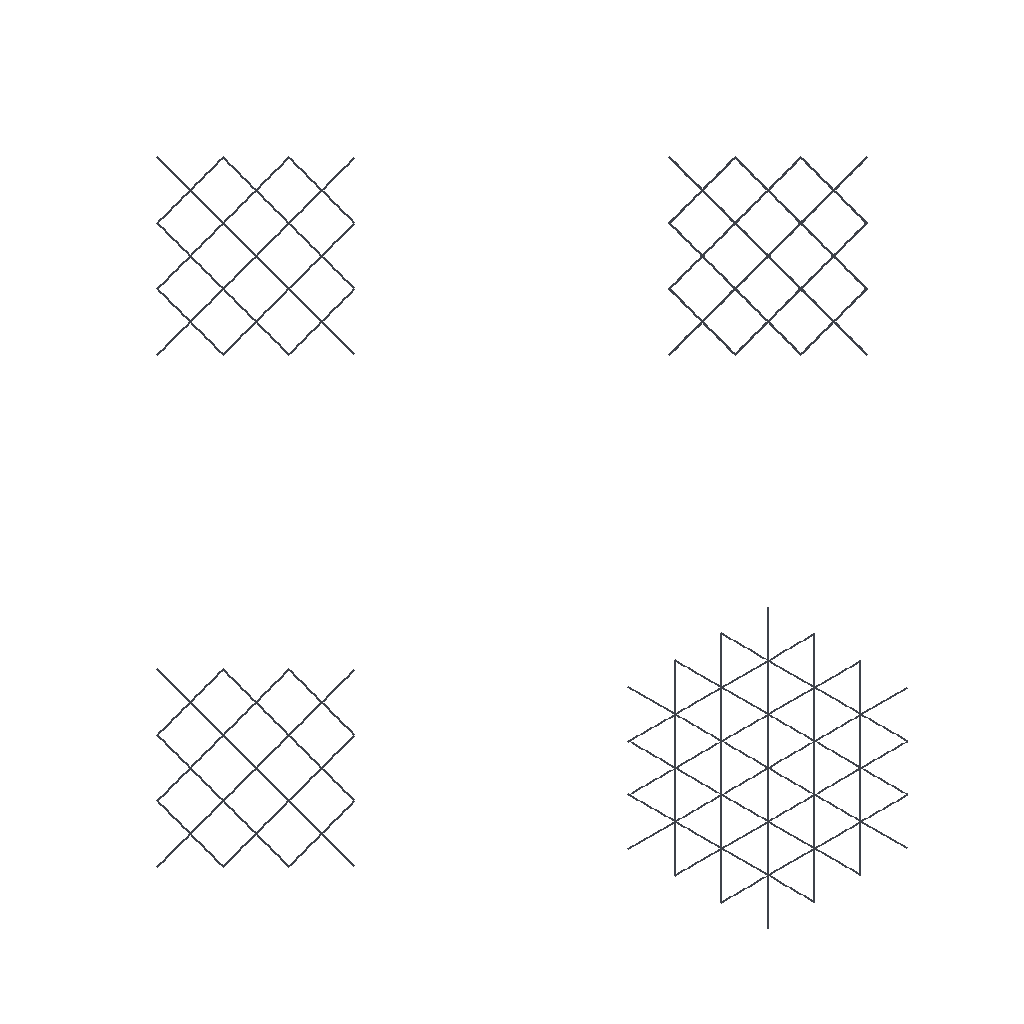Simulation study | abaqus
Set-up summary:
category,name,step,type,value,unit,region
solver,abaqus,,Abaqus/CAE 2024
units,mm-N-s-tonne (MPa),,inferred,E=90000 density=4.51e-09
analysis,Step-1,,dynamic explicit,nlgeom=True; time_period=0.002
mesh,nodes,,,2919
mesh,elements,,,2960
element_type,B31,,,2160
element_type,R3D4,,,800
material,Material-1,,E,90000
material,Material-1,,nu,0.3
material,Material-1,,density,4.51e-09
material,Material-1,,yield,782.7
material,Material-1,,behaviors,plastic; damage initiation; damage evolution
section,Material-1,,beam section,,,Set-1
bc,BC-1,initial,encastre,[dofs=ENCASTRE],,_PickedSet9
bc,BC-2,Step-1,fixed,"[dofs=rx,ry,rz,x,y n=5]",,_PickedSet10
bc,BC-2,Step-1,displacement,-5 [dofs=z],,_PickedSet10
contact,Int-1,initial,general contact,interaction=IntProp-1; friction=0.1; behavior=hard
constraint,rigid body,,,2
Abaqus input file, long lists of numbers shortened:
*Heading
** Job name: deck Model name: lingdian011
** Generated by: Abaqus/CAE 2024
*Preprint, echo=NO, model=NO, history=NO, contact=NO
**
** PARTS
**
*Part, name=BCC
*Node
      1,         12.5,         12.5,         12.5
      2,          10.,          10.,          15.
** (2033 more lines like these left out)
*Element, type=B31
 1,   1,  92
 2,  92,  93
** (2158 more lines like these left out)
*Nset, nset=Set-1, generate
    1,  2035,     1
*Elset, elset=Set-1, generate
    1,  2160,     1
** Section: Section-1  Profile: Profile-1
*Beam Section, elset=Set-1, material=Material-1, temperature=GRADIENTS, section=CIRC
0.11
0.,0.1,-1.
*End Part
**
*Part, name=Part-2
*Node
      1,         -10.,         -10.,           0.
      2,          -9.,         -10.,           0.
** (439 more lines like these left out)
*Element, type=R3D4
  1,   1,   2,  23,  22
  2,   2,   3,  24,  23
** (398 more lines like these left out)
*Node
    442,          10.,           0.,           0.
*Nset, nset=Part-2-RefPt_, internal
442,
*Elset, elset=Part-2, generate
   1,  400,    1
*End Part
**
**
** ASSEMBLY
**
*Assembly, name=Assembly
**
*Instance, name=BCC-1, part=BCC
        -7.5,         -7.5,           0.
*End Instance
**
*Instance, name=Part-2-1, part=Part-2
*End Instance
**
*Instance, name=Part-2-1-lin-2-1, part=Part-2
          0.,           0.,          15.
*End Instance
**
*Nset, nset=_PickedSet9, internal, instance=Part-2-1
 442,
*Nset, nset=_PickedSet10, internal, instance=Part-2-1-lin-2-1
 442,
*Rigid Body, ref node=Part-2-1.Part-2-RefPt_, elset=Part-2-1.Part-2
*Rigid Body, ref node=Part-2-1-lin-2-1.Part-2-RefPt_, elset=Part-2-1-lin-2-1.Part-2
*End Assembly
*Amplitude, name=Amp-1
             0.,              0.,           0.002,              1.
**
** MATERIALS
**
*Material, name=Material-1
*Damage Initiation, criterion=JOHNSON COOK
 -0.09, 0.25, -0.5,   0.,   0., 200., 100.,   1.
*Damage Evolution, type=DISPLACEMENT
1.,
*Density
 4.51e-09,
*Elastic
90000., 0.3
*Plastic, hardening=JOHNSON COOK
 782.7, 498.4,  0.28,    0.,  200.,  100.
**
** INTERACTION PROPERTIES
**
*Surface Interaction, name=IntProp-1
*Friction
 0.1,
*Surface Behavior, pressure-overclosure=HARD
**
** BOUNDARY CONDITIONS
**
** Name: BC-1 Type: Symmetry/Antisymmetry/Encastre
*Boundary
_PickedSet9, ENCASTRE
**
** INTERACTIONS
**
** Interaction: Int-1
*Contact, op=NEW
*Contact Inclusions, ALL EXTERIOR
*Contact Property Assignment
 ,  , IntProp-1
** ----------------------------------------------------------------
**
** STEP: Step-1
**
*Step, name=Step-1, nlgeom=YES
*Dynamic, Explicit
, 0.002
*Bulk Viscosity
0.06, 1.2
** Mass Scaling: Semi-Automatic
**               Whole Model
*Fixed Mass Scaling, factor=100.
**
** BOUNDARY CONDITIONS
**
** Name: BC-2 Type: Displacement/Rotation
*Boundary, amplitude=Amp-1
_PickedSet10, 1, 1
_PickedSet10, 2, 2
_PickedSet10, 3, 3, -5.
_PickedSet10, 4, 4
_PickedSet10, 5, 5
_PickedSet10, 6, 6
**
** OUTPUT REQUESTS
**
*Restart, write, number interval=1, time marks=NO
**
** FIELD OUTPUT: F-Output-1
**
*Output, field, variable=PRESELECT
**
** HISTORY OUTPUT: H-Output-1
**
*Output, history, variable=PRESELECT
*End Step
Results summary:
result,odb.job_status,,,JOB_STATUS_COMPLETED_SUCCESSFULLY,"consistent, unstated (Abaqus has no unit system)"
result,steps[0].procedure,Step-1,,"*DYNAMIC, EXPLICIT","consistent, unstated (Abaqus has no unit system)"
result,steps[0].time_period,Step-1,,0.002,"consistent, unstated (Abaqus has no unit system)"
result,steps[0].n_frames,Step-1,,21,"consistent, unstated (Abaqus has no unit system)"
result,steps[0].last_frame.id,Step-1,,3737,"consistent, unstated (Abaqus has no unit system)"
result,steps[0].last_frame.value,Step-1,,0.002,"consistent, unstated (Abaqus has no unit system)"
result,steps[0].last_frame.description,Step-1,,Increment      3737: Step Time =   2.0000E-03,"consistent, unstated (Abaqus has no unit system)"
result,steps[0].completed,Step-1,,True,"consistent, unstated (Abaqus has no unit system)"
result,steps[0].max_U_magnitude,Step-1,,5.303,"consistent, unstated (Abaqus has no unit system)"
result,steps[0].max_S_mises,Step-1,,1082.15,"consistent, unstated (Abaqus has no unit system)"
result,steps[0].RF_sum[1],Step-1,,0.5933,"consistent, unstated (Abaqus has no unit system)"
result,steps[0].RF_sum[2],Step-1,,0.8276,"consistent, unstated (Abaqus has no unit system)"
result,steps[0].RF_sum[3],Step-1,,15.799,"consistent, unstated (Abaqus has no unit system)"
result,steps[0].diagnostic.n_increments,Step-1,,21,"consistent, unstated (Abaqus has no unit system)"